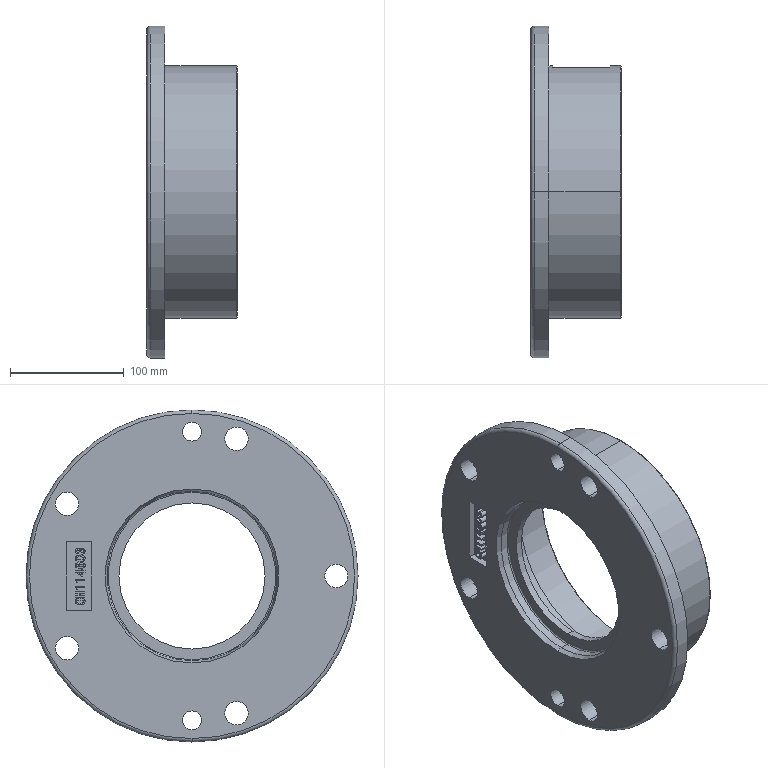Part | SolidWorks | features Fillet 5, ICE 4, HoleWzd 2, Chamfer 1, MirrorPattern 1, Revolution 1 | 1 solid | 156 faces | box 79.375 x 292.1 x 292.1 mm | volume 1441408 mm3 | plane 70 | spline 42 | cylinder 29 | torus 13 | cone 2 | commonest cylinder face diameters 20.637 x8 16.667 x4 6.096 x2 20.638 x2 128.524 x2 149.723 x2